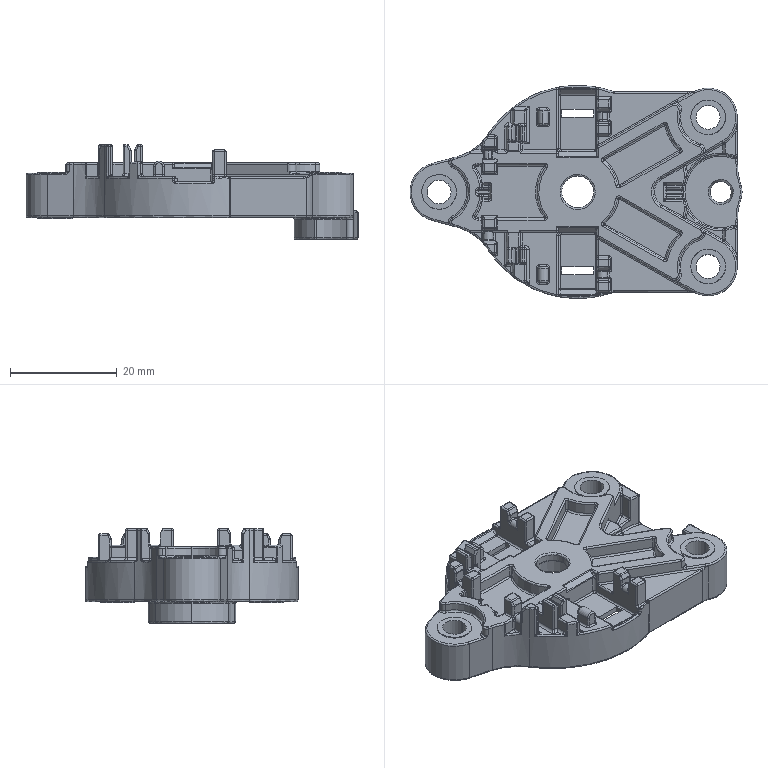Part | 1 solid | 1570 faces | box 62.36 x 40 x 17.8 mm | volume 10208 mm3 | spline 675 | cylinder 657 | plane 236 | cone 2 | commonest cylinder face diameters 0.6 x502 2 x27 1 x23 0.2 x12 6.5 x12 11 x11